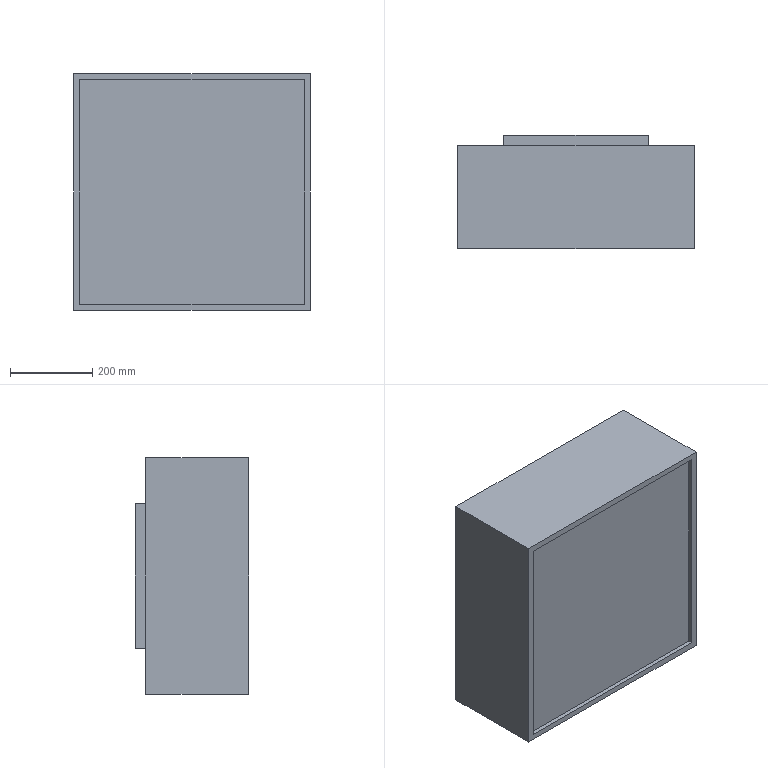Part | STEP file | FFU | 1 solid | 16 faces | box 575 x 275 x 575 mm | volume 82748500 mm3 | plane 16
STEP:
#1=CARTESIAN_POINT('',(0.,0.,0.));
#2=DIRECTION('',(0.,0.,1.));
#3=DIRECTION('',(1.,0.,0.));
#4=AXIS2_PLACEMENT_3D('',#1,#2,#3);
#5=CARTESIAN_POINT('',(-287.5,0.,-287.5));
#6=VERTEX_POINT('',#5);
#7=CARTESIAN_POINT('',(-287.5,0.,287.5));
#8=VERTEX_POINT('',#7);
#9=CARTESIAN_POINT('',(-287.5,0.,-287.5));
#10=DIRECTION('',(0.,0.,1.));
#11=VECTOR('',#10,1.);
#12=LINE('',#9,#11);
#13=CARTESIAN_POINT('',(-287.5,250.,-287.5));
#14=DIRECTION('',(1.,0.,0.));
#15=DIRECTION('',(0.,0.,-1.));
#16=AXIS2_PLACEMENT_3D('',#13,#14,#15);
#17=PLANE('',#16);
#18=CARTESIAN_POINT('',(0.,-250.));
#19=DIRECTION('',(-1.,0.));
#20=VECTOR('',#19,1.);
#21=LINE('',#18,#20);
#22=(GEOMETRIC_REPRESENTATION_CONTEXT(2)PARAMETRIC_REPRESENTATION_CONTEXT()REPRESENTATION_CONTEXT('',''));
#23=DEFINITIONAL_REPRESENTATION('',(#21),#22);
#24=PCURVE('',#17,#23);
#25=CARTESIAN_POINT('',(0.,0.,0.));
#26=DIRECTION('',(0.,1.,0.));
#27=DIRECTION('',(0.,0.,1.));
#28=AXIS2_PLACEMENT_3D('',#25,#26,#27);
#29=PLANE('',#28);
#30=CARTESIAN_POINT('',(-287.5,-287.5));
#31=DIRECTION('',(1.,0.));
#32=VECTOR('',#31,1.);
#33=LINE('',#30,#32);
#34=(GEOMETRIC_REPRESENTATION_CONTEXT(2)PARAMETRIC_REPRESENTATION_CONTEXT()REPRESENTATION_CONTEXT('',''));
#35=DEFINITIONAL_REPRESENTATION('',(#33),#34);
#36=PCURVE('',#29,#35);
#37=SURFACE_CURVE('',#12,(#24,#36),.PCURVE_S1.);
#38=EDGE_CURVE('',#6,#8,#37,.T.);
#39=ORIENTED_EDGE('',*,*,#38,.T.);
#40=CARTESIAN_POINT('',(-287.5,250.,287.5));
#41=VERTEX_POINT('',#40);
#42=CARTESIAN_POINT('',(-287.5,250.,287.5));
#43=DIRECTION('',(0.,-1.,0.));
#44=VECTOR('',#43,1.);
#45=LINE('',#42,#44);
#46=CARTESIAN_POINT('',(-575.,0.));
#47=DIRECTION('',(0.,-1.));
#48=VECTOR('',#47,1.);
#49=LINE('',#46,#48);
#50=(GEOMETRIC_REPRESENTATION_CONTEXT(2)PARAMETRIC_REPRESENTATION_CONTEXT()REPRESENTATION_CONTEXT('',''));
#51=DEFINITIONAL_REPRESENTATION('',(#49),#50);
#52=PCURVE('',#17,#51);
#53=CARTESIAN_POINT('',(-287.5,250.,287.5));
#54=DIRECTION('',(0.,0.,-1.));
#55=DIRECTION('',(-1.,0.,0.));
#56=AXIS2_PLACEMENT_3D('',#53,#54,#55);
#57=PLANE('',#56);
#58=CARTESIAN_POINT('',(0.,0.));
#59=DIRECTION('',(0.,-1.));
#60=VECTOR('',#59,1.);
#61=LINE('',#58,#60);
#62=(GEOMETRIC_REPRESENTATION_CONTEXT(2)PARAMETRIC_REPRESENTATION_CONTEXT()REPRESENTATION_CONTEXT('',''));
#63=DEFINITIONAL_REPRESENTATION('',(#61),#62);
#64=PCURVE('',#57,#63);
#65=SURFACE_CURVE('',#45,(#52,#64),.PCURVE_S1.);
#66=EDGE_CURVE('',#41,#8,#65,.T.);
#67=ORIENTED_EDGE('',*,*,#66,.F.);
#68=CARTESIAN_POINT('',(-287.5,250.,-287.5));
#69=VERTEX_POINT('',#68);
#70=CARTESIAN_POINT('',(-287.5,250.,-287.5));
#71=DIRECTION('',(0.,0.,1.));
#72=VECTOR('',#71,1.);
#73=LINE('',#70,#72);
#74=CARTESIAN_POINT('',(0.,0.));
#75=DIRECTION('',(-1.,0.));
#76=VECTOR('',#75,1.);
#77=LINE('',#74,#76);
#78=(GEOMETRIC_REPRESENTATION_CONTEXT(2)PARAMETRIC_REPRESENTATION_CONTEXT()REPRESENTATION_CONTEXT('',''));
#79=DEFINITIONAL_REPRESENTATION('',(#77),#78);
#80=PCURVE('',#17,#79);
#81=CARTESIAN_POINT('',(0.,250.,0.));
#82=DIRECTION('',(0.,1.,0.));
#83=DIRECTION('',(0.,0.,1.));
#84=AXIS2_PLACEMENT_3D('',#81,#82,#83);
#85=PLANE('',#84);
#86=CARTESIAN_POINT('',(-287.5,-287.5));
#87=DIRECTION('',(1.,0.));
#88=VECTOR('',#87,1.);
#89=LINE('',#86,#88);
#90=(GEOMETRIC_REPRESENTATION_CONTEXT(2)PARAMETRIC_REPRESENTATION_CONTEXT()REPRESENTATION_CONTEXT('',''));
#91=DEFINITIONAL_REPRESENTATION('',(#89),#90);
#92=PCURVE('',#85,#91);
#93=SURFACE_CURVE('',#73,(#80,#92),.PCURVE_S1.);
#94=EDGE_CURVE('',#69,#41,#93,.T.);
#95=ORIENTED_EDGE('',*,*,#94,.F.);
#96=CARTESIAN_POINT('',(-287.5,250.,-287.5));
#97=DIRECTION('',(0.,-1.,0.));
#98=VECTOR('',#97,1.);
#99=LINE('',#96,#98);
#100=CARTESIAN_POINT('',(0.,0.));
#101=DIRECTION('',(0.,-1.));
#102=VECTOR('',#101,1.);
#103=LINE('',#100,#102);
#104=(GEOMETRIC_REPRESENTATION_CONTEXT(2)PARAMETRIC_REPRESENTATION_CONTEXT()REPRESENTATION_CONTEXT('',''));
#105=DEFINITIONAL_REPRESENTATION('',(#103),#104);
#106=PCURVE('',#17,#105);
#107=CARTESIAN_POINT('',(-287.5,250.,-287.5));
#108=DIRECTION('',(0.,0.,1.));
#109=DIRECTION('',(1.,0.,0.));
#110=AXIS2_PLACEMENT_3D('',#107,#108,#109);
#111=PLANE('',#110);
#112=CARTESIAN_POINT('',(0.,0.));
#113=DIRECTION('',(0.,-1.));
#114=VECTOR('',#113,1.);
#115=LINE('',#112,#114);
#116=(GEOMETRIC_REPRESENTATION_CONTEXT(2)PARAMETRIC_REPRESENTATION_CONTEXT()REPRESENTATION_CONTEXT('',''));
#117=DEFINITIONAL_REPRESENTATION('',(#115),#116);
#118=PCURVE('',#111,#117);
#119=SURFACE_CURVE('',#99,(#106,#118),.PCURVE_S1.);
#120=EDGE_CURVE('',#69,#6,#119,.T.);
#121=ORIENTED_EDGE('',*,*,#120,.T.);
#122=EDGE_LOOP('',(#39,#67,#95,#121));
#123=FACE_BOUND('',#122,.T.);
#124=ADVANCED_FACE('',(#123),#17,.F.);
#125=CARTESIAN_POINT('',(287.5,0.,287.5));
#126=VERTEX_POINT('',#125);
#127=CARTESIAN_POINT('',(-287.5,0.,287.5));
#128=DIRECTION('',(1.,0.,0.));
#129=VECTOR('',#128,1.);
#130=LINE('',#127,#129);
#131=CARTESIAN_POINT('',(0.,-250.));
#132=DIRECTION('',(-1.,0.));
#133=VECTOR('',#132,1.);
#134=LINE('',#131,#133);
#135=(GEOMETRIC_REPRESENTATION_CONTEXT(2)PARAMETRIC_REPRESENTATION_CONTEXT()REPRESENTATION_CONTEXT('',''));
#136=DEFINITIONAL_REPRESENTATION('',(#134),#135);
#137=PCURVE('',#57,#136);
#138=CARTESIAN_POINT('',(287.5,-287.5));
#139=DIRECTION('',(0.,1.));
#140=VECTOR('',#139,1.);
#141=LINE('',#138,#140);
#142=(GEOMETRIC_REPRESENTATION_CONTEXT(2)PARAMETRIC_REPRESENTATION_CONTEXT()REPRESENTATION_CONTEXT('',''));
#143=DEFINITIONAL_REPRESENTATION('',(#141),#142);
#144=PCURVE('',#29,#143);
#145=SURFACE_CURVE('',#130,(#137,#144),.PCURVE_S1.);
#146=EDGE_CURVE('',#8,#126,#145,.T.);
#147=ORIENTED_EDGE('',*,*,#146,.T.);
#148=CARTESIAN_POINT('',(287.5,250.,287.5));
#149=VERTEX_POINT('',#148);
#150=CARTESIAN_POINT('',(287.5,250.,287.5));
#151=DIRECTION('',(0.,-1.,0.));
#152=VECTOR('',#151,1.);
#153=LINE('',#150,#152);
#154=CARTESIAN_POINT('',(-575.,0.));
#155=DIRECTION('',(0.,-1.));
#156=VECTOR('',#155,1.);
#157=LINE('',#154,#156);
#158=(GEOMETRIC_REPRESENTATION_CONTEXT(2)PARAMETRIC_REPRESENTATION_CONTEXT()REPRESENTATION_CONTEXT('',''));
#159=DEFINITIONAL_REPRESENTATION('',(#157),#158);
#160=PCURVE('',#57,#159);
#161=CARTESIAN_POINT('',(287.5,250.,-287.5));
#162=DIRECTION('',(-1.,0.,0.));
#163=DIRECTION('',(0.,0.,1.));
#164=AXIS2_PLACEMENT_3D('',#161,#162,#163);
#165=PLANE('',#164);
#166=CARTESIAN_POINT('',(575.,0.));
#167=DIRECTION('',(0.,-1.));
#168=VECTOR('',#167,1.);
#169=LINE('',#166,#168);
#170=(GEOMETRIC_REPRESENTATION_CONTEXT(2)PARAMETRIC_REPRESENTATION_CONTEXT()REPRESENTATION_CONTEXT('',''));
#171=DEFINITIONAL_REPRESENTATION('',(#169),#170);
#172=PCURVE('',#165,#171);
#173=SURFACE_CURVE('',#153,(#160,#172),.PCURVE_S1.);
#174=EDGE_CURVE('',#149,#126,#173,.T.);
#175=ORIENTED_EDGE('',*,*,#174,.F.);
#176=CARTESIAN_POINT('',(-287.5,250.,287.5));
#177=DIRECTION('',(1.,0.,0.));
#178=VECTOR('',#177,1.);
#179=LINE('',#176,#178);
#180=CARTESIAN_POINT('',(0.,0.));
#181=DIRECTION('',(-1.,0.));
#182=VECTOR('',#181,1.);
#183=LINE('',#180,#182);
#184=(GEOMETRIC_REPRESENTATION_CONTEXT(2)PARAMETRIC_REPRESENTATION_CONTEXT()REPRESENTATION_CONTEXT('',''));
#185=DEFINITIONAL_REPRESENTATION('',(#183),#184);
#186=PCURVE('',#57,#185);
#187=CARTESIAN_POINT('',(287.5,-287.5));
#188=DIRECTION('',(0.,1.));
#189=VECTOR('',#188,1.);
#190=LINE('',#187,#189);
#191=(GEOMETRIC_REPRESENTATION_CONTEXT(2)PARAMETRIC_REPRESENTATION_CONTEXT()REPRESENTATION_CONTEXT('',''));
#192=DEFINITIONAL_REPRESENTATION('',(#190),#191);
#193=PCURVE('',#85,#192);
#194=SURFACE_CURVE('',#179,(#186,#193),.PCURVE_S1.);
#195=EDGE_CURVE('',#41,#149,#194,.T.);
#196=ORIENTED_EDGE('',*,*,#195,.F.);
#197=ORIENTED_EDGE('',*,*,#66,.T.);
#198=EDGE_LOOP('',(#147,#175,#196,#197));
#199=FACE_BOUND('',#198,.T.);
#200=ADVANCED_FACE('',(#199),#57,.F.);
#201=CARTESIAN_POINT('',(287.5,0.,-287.5));
#202=VERTEX_POINT('',#201);
#203=CARTESIAN_POINT('',(287.5,0.,-287.5));
#204=DIRECTION('',(0.,0.,-1.));
#205=VECTOR('',#204,1.);
#206=LINE('',#203,#205);
#207=CARTESIAN_POINT('',(0.,-250.));
#208=DIRECTION('',(-1.,0.));
#209=VECTOR('',#208,1.);
#210=LINE('',#207,#209);
#211=(GEOMETRIC_REPRESENTATION_CONTEXT(2)PARAMETRIC_REPRESENTATION_CONTEXT()REPRESENTATION_CONTEXT('',''));
#212=DEFINITIONAL_REPRESENTATION('',(#210),#211);
#213=PCURVE('',#165,#212);
#214=CARTESIAN_POINT('',(-287.5,287.5));
#215=DIRECTION('',(-1.,0.));
#216=VECTOR('',#215,1.);
#217=LINE('',#214,#216);
#218=(GEOMETRIC_REPRESENTATION_CONTEXT(2)PARAMETRIC_REPRESENTATION_CONTEXT()REPRESENTATION_CONTEXT('',''));
#219=DEFINITIONAL_REPRESENTATION('',(#217),#218);
#220=PCURVE('',#29,#219);
#221=SURFACE_CURVE('',#206,(#213,#220),.PCURVE_S1.);
#222=EDGE_CURVE('',#126,#202,#221,.T.);
#223=ORIENTED_EDGE('',*,*,#222,.T.);
#224=CARTESIAN_POINT('',(287.5,250.,-287.5));
#225=VERTEX_POINT('',#224);
#226=CARTESIAN_POINT('',(287.5,250.,-287.5));
#227=DIRECTION('',(0.,-1.,0.));
#228=VECTOR('',#227,1.);
#229=LINE('',#226,#228);
#230=CARTESIAN_POINT('',(0.,0.));
#231=DIRECTION('',(0.,-1.));
#232=VECTOR('',#231,1.);
#233=LINE('',#230,#232);
#234=(GEOMETRIC_REPRESENTATION_CONTEXT(2)PARAMETRIC_REPRESENTATION_CONTEXT()REPRESENTATION_CONTEXT('',''));
#235=DEFINITIONAL_REPRESENTATION('',(#233),#234);
#236=PCURVE('',#165,#235);
#237=CARTESIAN_POINT('',(575.,0.));
#238=DIRECTION('',(0.,-1.));
#239=VECTOR('',#238,1.);
#240=LINE('',#237,#239);
#241=(GEOMETRIC_REPRESENTATION_CONTEXT(2)PARAMETRIC_REPRESENTATION_CONTEXT()REPRESENTATION_CONTEXT('',''));
#242=DEFINITIONAL_REPRESENTATION('',(#240),#241);
#243=PCURVE('',#111,#242);
#244=SURFACE_CURVE('',#229,(#236,#243),.PCURVE_S1.);
#245=EDGE_CURVE('',#225,#202,#244,.T.);
#246=ORIENTED_EDGE('',*,*,#245,.F.);
#247=CARTESIAN_POINT('',(287.5,250.,-287.5));
#248=DIRECTION('',(0.,0.,-1.));
#249=VECTOR('',#248,1.);
#250=LINE('',#247,#249);
#251=CARTESIAN_POINT('',(0.,0.));
#252=DIRECTION('',(-1.,0.));
#253=VECTOR('',#252,1.);
#254=LINE('',#251,#253);
#255=(GEOMETRIC_REPRESENTATION_CONTEXT(2)PARAMETRIC_REPRESENTATION_CONTEXT()REPRESENTATION_CONTEXT('',''));
#256=DEFINITIONAL_REPRESENTATION('',(#254),#255);
#257=PCURVE('',#165,#256);
#258=CARTESIAN_POINT('',(-287.5,287.5));
#259=DIRECTION('',(-1.,0.));
#260=VECTOR('',#259,1.);
#261=LINE('',#258,#260);
#262=(GEOMETRIC_REPRESENTATION_CONTEXT(2)PARAMETRIC_REPRESENTATION_CONTEXT()REPRESENTATION_CONTEXT('',''));
#263=DEFINITIONAL_REPRESENTATION('',(#261),#262);
#264=PCURVE('',#85,#263);
#265=SURFACE_CURVE('',#250,(#257,#264),.PCURVE_S1.);
#266=EDGE_CURVE('',#149,#225,#265,.T.);
#267=ORIENTED_EDGE('',*,*,#266,.F.);
#268=ORIENTED_EDGE('',*,*,#174,.T.);
#269=EDGE_LOOP('',(#223,#246,#267,#268));
#270=FACE_BOUND('',#269,.T.);
#271=ADVANCED_FACE('',(#270),#165,.F.);
#272=CARTESIAN_POINT('',(-287.5,0.,-287.5));
#273=DIRECTION('',(-1.,0.,0.));
#274=VECTOR('',#273,1.);
#275=LINE('',#272,#274);
#276=CARTESIAN_POINT('',(0.,-250.));
#277=DIRECTION('',(-1.,0.));
#278=VECTOR('',#277,1.);
#279=LINE('',#276,#278);
#280=(GEOMETRIC_REPRESENTATION_CONTEXT(2)PARAMETRIC_REPRESENTATION_CONTEXT()REPRESENTATION_CONTEXT('',''));
#281=DEFINITIONAL_REPRESENTATION('',(#279),#280);
#282=PCURVE('',#111,#281);
#283=CARTESIAN_POINT('',(-287.5,-287.5));
#284=DIRECTION('',(0.,-1.));
#285=VECTOR('',#284,1.);
#286=LINE('',#283,#285);
#287=(GEOMETRIC_REPRESENTATION_CONTEXT(2)PARAMETRIC_REPRESENTATION_CONTEXT()REPRESENTATION_CONTEXT('',''));
#288=DEFINITIONAL_REPRESENTATION('',(#286),#287);
#289=PCURVE('',#29,#288);
#290=SURFACE_CURVE('',#275,(#282,#289),.PCURVE_S1.);
#291=EDGE_CURVE('',#202,#6,#290,.T.);
#292=ORIENTED_EDGE('',*,*,#291,.T.);
#293=ORIENTED_EDGE('',*,*,#120,.F.);
#294=CARTESIAN_POINT('',(-287.5,250.,-287.5));
#295=DIRECTION('',(-1.,0.,0.));
#296=VECTOR('',#295,1.);
#297=LINE('',#294,#296);
#298=CARTESIAN_POINT('',(0.,0.));
#299=DIRECTION('',(-1.,0.));
#300=VECTOR('',#299,1.);
#301=LINE('',#298,#300);
#302=(GEOMETRIC_REPRESENTATION_CONTEXT(2)PARAMETRIC_REPRESENTATION_CONTEXT()REPRESENTATION_CONTEXT('',''));
#303=DEFINITIONAL_REPRESENTATION('',(#301),#302);
#304=PCURVE('',#111,#303);
#305=CARTESIAN_POINT('',(-287.5,-287.5));
#306=DIRECTION('',(0.,-1.));
#307=VECTOR('',#306,1.);
#308=LINE('',#305,#307);
#309=(GEOMETRIC_REPRESENTATION_CONTEXT(2)PARAMETRIC_REPRESENTATION_CONTEXT()REPRESENTATION_CONTEXT('',''));
#310=DEFINITIONAL_REPRESENTATION('',(#308),#309);
#311=PCURVE('',#85,#310);
#312=SURFACE_CURVE('',#297,(#304,#311),.PCURVE_S1.);
#313=EDGE_CURVE('',#225,#69,#312,.T.);
#314=ORIENTED_EDGE('',*,*,#313,.F.);
#315=ORIENTED_EDGE('',*,*,#245,.T.);
#316=EDGE_LOOP('',(#292,#293,#314,#315));
#317=FACE_BOUND('',#316,.T.);
#318=ADVANCED_FACE('',(#317),#111,.F.);
#319=CARTESIAN_POINT('',(175.,250.,175.));
#320=VERTEX_POINT('',#319);
#321=CARTESIAN_POINT('',(175.,250.,-175.));
#322=VERTEX_POINT('',#321);
#323=CARTESIAN_POINT('',(175.,250.,175.));
#324=DIRECTION('',(0.,0.,-1.));
#325=VECTOR('',#324,1.);
#326=LINE('',#323,#325);
#327=CARTESIAN_POINT('',(175.,175.));
#328=DIRECTION('',(-1.,0.));
#329=VECTOR('',#328,1.);
#330=LINE('',#327,#329);
#331=(GEOMETRIC_REPRESENTATION_CONTEXT(2)PARAMETRIC_REPRESENTATION_CONTEXT()REPRESENTATION_CONTEXT('',''));
#332=DEFINITIONAL_REPRESENTATION('',(#330),#331);
#333=PCURVE('',#85,#332);
#334=CARTESIAN_POINT('',(175.,275.,175.));
#335=DIRECTION('',(-1.,0.,0.));
#336=DIRECTION('',(0.,0.,1.));
#337=AXIS2_PLACEMENT_3D('',#334,#335,#336);
#338=PLANE('',#337);
#339=CARTESIAN_POINT('',(0.,-25.));
#340=DIRECTION('',(-1.,0.));
#341=VECTOR('',#340,1.);
#342=LINE('',#339,#341);
#343=(GEOMETRIC_REPRESENTATION_CONTEXT(2)PARAMETRIC_REPRESENTATION_CONTEXT()REPRESENTATION_CONTEXT('',''));
#344=DEFINITIONAL_REPRESENTATION('',(#342),#343);
#345=PCURVE('',#338,#344);
#346=SURFACE_CURVE('',#326,(#333,#345),.PCURVE_S1.);
#347=EDGE_CURVE('',#320,#322,#346,.T.);
#348=ORIENTED_EDGE('',*,*,#347,.F.);
#349=CARTESIAN_POINT('',(-175.,250.,175.));
#350=VERTEX_POINT('',#349);
#351=CARTESIAN_POINT('',(-175.,250.,175.));
#352=DIRECTION('',(1.,0.,0.));
#353=VECTOR('',#352,1.);
#354=LINE('',#351,#353);
#355=CARTESIAN_POINT('',(175.,-175.));
#356=DIRECTION('',(0.,1.));
#357=VECTOR('',#356,1.);
#358=LINE('',#355,#357);
#359=(GEOMETRIC_REPRESENTATION_CONTEXT(2)PARAMETRIC_REPRESENTATION_CONTEXT()REPRESENTATION_CONTEXT('',''));
#360=DEFINITIONAL_REPRESENTATION('',(#358),#359);
#361=PCURVE('',#85,#360);
#362=CARTESIAN_POINT('',(-175.,275.,175.));
#363=DIRECTION('',(0.,0.,-1.));
#364=DIRECTION('',(0.,1.,0.));
#365=AXIS2_PLACEMENT_3D('',#362,#363,#364);
#366=PLANE('',#365);
#367=CARTESIAN_POINT('',(-25.,0.));
#368=DIRECTION('',(0.,1.));
#369=VECTOR('',#368,1.);
#370=LINE('',#367,#369);
#371=(GEOMETRIC_REPRESENTATION_CONTEXT(2)PARAMETRIC_REPRESENTATION_CONTEXT()REPRESENTATION_CONTEXT('',''));
#372=DEFINITIONAL_REPRESENTATION('',(#370),#371);
#373=PCURVE('',#366,#372);
#374=SURFACE_CURVE('',#354,(#361,#373),.PCURVE_S1.);
#375=EDGE_CURVE('',#350,#320,#374,.T.);
#376=ORIENTED_EDGE('',*,*,#375,.F.);
#377=CARTESIAN_POINT('',(-175.,250.,-175.));
#378=VERTEX_POINT('',#377);
#379=CARTESIAN_POINT('',(-175.,250.,175.));
#380=DIRECTION('',(0.,0.,1.));
#381=VECTOR('',#380,1.);
#382=LINE('',#379,#381);
#383=CARTESIAN_POINT('',(175.,-175.));
#384=DIRECTION('',(1.,0.));
#385=VECTOR('',#384,1.);
#386=LINE('',#383,#385);
#387=(GEOMETRIC_REPRESENTATION_CONTEXT(2)PARAMETRIC_REPRESENTATION_CONTEXT()REPRESENTATION_CONTEXT('',''));
#388=DEFINITIONAL_REPRESENTATION('',(#386),#387);
#389=PCURVE('',#85,#388);
#390=CARTESIAN_POINT('',(-175.,275.,175.));
#391=DIRECTION('',(1.,0.,0.));
#392=DIRECTION('',(0.,0.,-1.));
#393=AXIS2_PLACEMENT_3D('',#390,#391,#392);
#394=PLANE('',#393);
#395=CARTESIAN_POINT('',(0.,-25.));
#396=DIRECTION('',(-1.,0.));
#397=VECTOR('',#396,1.);
#398=LINE('',#395,#397);
#399=(GEOMETRIC_REPRESENTATION_CONTEXT(2)PARAMETRIC_REPRESENTATION_CONTEXT()REPRESENTATION_CONTEXT('',''));
#400=DEFINITIONAL_REPRESENTATION('',(#398),#399);
#401=PCURVE('',#394,#400);
#402=SURFACE_CURVE('',#382,(#389,#401),.PCURVE_S1.);
#403=EDGE_CURVE('',#378,#350,#402,.T.);
#404=ORIENTED_EDGE('',*,*,#403,.F.);
#405=CARTESIAN_POINT('',(-175.,250.,-175.));
#406=DIRECTION('',(-1.,0.,0.));
#407=VECTOR('',#406,1.);
#408=LINE('',#405,#407);
#409=CARTESIAN_POINT('',(-175.,-175.));
#410=DIRECTION('',(0.,-1.));
#411=VECTOR('',#410,1.);
#412=LINE('',#409,#411);
#413=(GEOMETRIC_REPRESENTATION_CONTEXT(2)PARAMETRIC_REPRESENTATION_CONTEXT()REPRESENTATION_CONTEXT('',''));
#414=DEFINITIONAL_REPRESENTATION('',(#412),#413);
#415=PCURVE('',#85,#414);
#416=CARTESIAN_POINT('',(-175.,275.,-175.));
#417=DIRECTION('',(0.,0.,1.));
#418=DIRECTION('',(0.,-1.,0.));
#419=AXIS2_PLACEMENT_3D('',#416,#417,#418);
#420=PLANE('',#419);
#421=CARTESIAN_POINT('',(25.,0.));
#422=DIRECTION('',(0.,-1.));
#423=VECTOR('',#422,1.);
#424=LINE('',#421,#423);
#425=(GEOMETRIC_REPRESENTATION_CONTEXT(2)PARAMETRIC_REPRESENTATION_CONTEXT()REPRESENTATION_CONTEXT('',''));
#426=DEFINITIONAL_REPRESENTATION('',(#424),#425);
#427=PCURVE('',#420,#426);
#428=SURFACE_CURVE('',#408,(#415,#427),.PCURVE_S1.);
#429=EDGE_CURVE('',#322,#378,#428,.T.);
#430=ORIENTED_EDGE('',*,*,#429,.F.);
#431=EDGE_LOOP('',(#348,#376,#404,#430));
#432=FACE_BOUND('',#431,.T.);
#433=ORIENTED_EDGE('',*,*,#94,.T.);
#434=ORIENTED_EDGE('',*,*,#195,.T.);
#435=ORIENTED_EDGE('',*,*,#266,.T.);
#436=ORIENTED_EDGE('',*,*,#313,.T.);
#437=EDGE_LOOP('',(#433,#434,#435,#436));
#438=FACE_BOUND('',#437,.T.);
#439=ADVANCED_FACE('',(#432,#438),#85,.T.);
#440=CARTESIAN_POINT('',(-272.5,0.,-272.5));
#441=VERTEX_POINT('',#440);
#442=CARTESIAN_POINT('',(272.5,0.,-272.5));
#443=VERTEX_POINT('',#442);
#444=CARTESIAN_POINT('',(-272.5,0.,-272.5));
#445=DIRECTION('',(1.,0.,0.));
#446=VECTOR('',#445,1.);
#447=LINE('',#444,#446);
#448=CARTESIAN_POINT('',(-272.5,-272.5));
#449=DIRECTION('',(0.,1.));
#450=VECTOR('',#449,1.);
#451=LINE('',#448,#450);
#452=(GEOMETRIC_REPRESENTATION_CONTEXT(2)PARAMETRIC_REPRESENTATION_CONTEXT()REPRESENTATION_CONTEXT('',''));
#453=DEFINITIONAL_REPRESENTATION('',(#451),#452);
#454=PCURVE('',#29,#453);
#455=CARTESIAN_POINT('',(-272.5,10.,-272.5));
#456=DIRECTION('',(0.,0.,-1.));
#457=DIRECTION('',(-1.,0.,0.));
#458=AXIS2_PLACEMENT_3D('',#455,#456,#457);
#459=PLANE('',#458);
#460=CARTESIAN_POINT('',(0.,-10.));
#461=DIRECTION('',(-1.,0.));
#462=VECTOR('',#461,1.);
#463=LINE('',#460,#462);
#464=(GEOMETRIC_REPRESENTATION_CONTEXT(2)PARAMETRIC_REPRESENTATION_CONTEXT()REPRESENTATION_CONTEXT('',''));
#465=DEFINITIONAL_REPRESENTATION('',(#463),#464);
#466=PCURVE('',#459,#465);
#467=SURFACE_CURVE('',#447,(#454,#466),.PCURVE_S1.);
#468=EDGE_CURVE('',#441,#443,#467,.T.);
#469=ORIENTED_EDGE('',*,*,#468,.F.);
#470=CARTESIAN_POINT('',(-272.5,0.,272.5));
#471=VERTEX_POINT('',#470);
#472=CARTESIAN_POINT('',(-272.5,0.,272.5));
#473=DIRECTION('',(0.,0.,-1.));
#474=VECTOR('',#473,1.);
#475=LINE('',#472,#474);
#476=CARTESIAN_POINT('',(272.5,-272.5));
#477=DIRECTION('',(-1.,0.));
#478=VECTOR('',#477,1.);
#479=LINE('',#476,#478);
#480=(GEOMETRIC_REPRESENTATION_CONTEXT(2)PARAMETRIC_REPRESENTATION_CONTEXT()REPRESENTATION_CONTEXT('',''));
#481=DEFINITIONAL_REPRESENTATION('',(#479),#480);
#482=PCURVE('',#29,#481);
#483=CARTESIAN_POINT('',(-272.5,10.,272.5));
#484=DIRECTION('',(-1.,0.,0.));
#485=DIRECTION('',(0.,0.,1.));
#486=AXIS2_PLACEMENT_3D('',#483,#484,#485);
#487=PLANE('',#486);
#488=CARTESIAN_POINT('',(0.,-10.));
#489=DIRECTION('',(-1.,0.));
#490=VECTOR('',#489,1.);
#491=LINE('',#488,#490);
#492=(GEOMETRIC_REPRESENTATION_CONTEXT(2)PARAMETRIC_REPRESENTATION_CONTEXT()REPRESENTATION_CONTEXT('',''));
#493=DEFINITIONAL_REPRESENTATION('',(#491),#492);
#494=PCURVE('',#487,#493);
#495=SURFACE_CURVE('',#475,(#482,#494),.PCURVE_S1.);
#496=EDGE_CURVE('',#471,#441,#495,.T.);
#497=ORIENTED_EDGE('',*,*,#496,.F.);
#498=CARTESIAN_POINT('',(272.5,0.,272.5));
#499=VERTEX_POINT('',#498);
#500=CARTESIAN_POINT('',(-272.5,0.,272.5));
#501=DIRECTION('',(-1.,0.,0.));
#502=VECTOR('',#501,1.);
#503=LINE('',#500,#502);
#504=CARTESIAN_POINT('',(272.5,-272.5));
#505=DIRECTION('',(0.,-1.));
#506=VECTOR('',#505,1.);
#507=LINE('',#504,#506);
#508=(GEOMETRIC_REPRESENTATION_CONTEXT(2)PARAMETRIC_REPRESENTATION_CONTEXT()REPRESENTATION_CONTEXT('',''));
#509=DEFINITIONAL_REPRESENTATION('',(#507),#508);
#510=PCURVE('',#29,#509);
#511=CARTESIAN_POINT('',(-272.5,10.,272.5));
#512=DIRECTION('',(0.,0.,1.));
#513=DIRECTION('',(1.,0.,0.));
#514=AXIS2_PLACEMENT_3D('',#511,#512,#513);
#515=PLANE('',#514);
#516=CARTESIAN_POINT('',(0.,-10.));
#517=DIRECTION('',(-1.,0.));
#518=VECTOR('',#517,1.);
#519=LINE('',#516,#518);
#520=(GEOMETRIC_REPRESENTATION_CONTEXT(2)PARAMETRIC_REPRESENTATION_CONTEXT()REPRESENTATION_CONTEXT('',''));
#521=DEFINITIONAL_REPRESENTATION('',(#519),#520);
#522=PCURVE('',#515,#521);
#523=SURFACE_CURVE('',#503,(#510,#522),.PCURVE_S1.);
#524=EDGE_CURVE('',#499,#471,#523,.T.);
#525=ORIENTED_EDGE('',*,*,#524,.F.);
#526=CARTESIAN_POINT('',(272.5,0.,272.5));
#527=DIRECTION('',(0.,0.,1.));
#528=VECTOR('',#527,1.);
#529=LINE('',#526,#528);
#530=CARTESIAN_POINT('',(272.5,272.5));
#531=DIRECTION('',(1.,0.));
#532=VECTOR('',#531,1.);
#533=LINE('',#530,#532);
#534=(GEOMETRIC_REPRESENTATION_CONTEXT(2)PARAMETRIC_REPRESENTATION_CONTEXT()REPRESENTATION_CONTEXT('',''));
#535=DEFINITIONAL_REPRESENTATION('',(#533),#534);
#536=PCURVE('',#29,#535);
#537=CARTESIAN_POINT('',(272.5,10.,272.5));
#538=DIRECTION('',(1.,0.,0.));
#539=DIRECTION('',(0.,0.,-1.));
#540=AXIS2_PLACEMENT_3D('',#537,#538,#539);
#541=PLANE('',#540);
#542=CARTESIAN_POINT('',(0.,-10.));
#543=DIRECTION('',(-1.,0.));
#544=VECTOR('',#543,1.);
#545=LINE('',#542,#544);
#546=(GEOMETRIC_REPRESENTATION_CONTEXT(2)PARAMETRIC_REPRESENTATION_CONTEXT()REPRESENTATION_CONTEXT('',''));
#547=DEFINITIONAL_REPRESENTATION('',(#545),#546);
#548=PCURVE('',#541,#547);
#549=SURFACE_CURVE('',#529,(#536,#548),.PCURVE_S1.);
#550=EDGE_CURVE('',#443,#499,#549,.T.);
#551=ORIENTED_EDGE('',*,*,#550,.F.);
#552=EDGE_LOOP('',(#469,#497,#525,#551));
#553=FACE_BOUND('',#552,.T.);
#554=ORIENTED_EDGE('',*,*,#38,.F.);
#555=ORIENTED_EDGE('',*,*,#291,.F.);
#556=ORIENTED_EDGE('',*,*,#222,.F.);
#557=ORIENTED_EDGE('',*,*,#146,.F.);
#558=EDGE_LOOP('',(#554,#555,#556,#557));
#559=FACE_BOUND('',#558,.T.);
#560=ADVANCED_FACE('',(#553,#559),#29,.F.);
#561=ORIENTED_EDGE('',*,*,#496,.T.);
#562=CARTESIAN_POINT('',(-272.5,10.,-272.5));
#563=VERTEX_POINT('',#562);
#564=CARTESIAN_POINT('',(-272.5,10.,-272.5));
#565=DIRECTION('',(0.,-1.,0.));
#566=VECTOR('',#565,1.);
#567=LINE('',#564,#566);
#568=CARTESIAN_POINT('',(-545.,0.));
#569=DIRECTION('',(0.,-1.));
#570=VECTOR('',#569,1.);
#571=LINE('',#568,#570);
#572=(GEOMETRIC_REPRESENTATION_CONTEXT(2)PARAMETRIC_REPRESENTATION_CONTEXT()REPRESENTATION_CONTEXT('',''));
#573=DEFINITIONAL_REPRESENTATION('',(#571),#572);
#574=PCURVE('',#487,#573);
#575=CARTESIAN_POINT('',(0.,0.));
#576=DIRECTION('',(0.,-1.));
#577=VECTOR('',#576,1.);
#578=LINE('',#575,#577);
#579=(GEOMETRIC_REPRESENTATION_CONTEXT(2)PARAMETRIC_REPRESENTATION_CONTEXT()REPRESENTATION_CONTEXT('',''));
#580=DEFINITIONAL_REPRESENTATION('',(#578),#579);
#581=PCURVE('',#459,#580);
#582=SURFACE_CURVE('',#567,(#574,#581),.PCURVE_S1.);
#583=EDGE_CURVE('',#563,#441,#582,.T.);
#584=ORIENTED_EDGE('',*,*,#583,.F.);
#585=CARTESIAN_POINT('',(-272.5,10.,272.5));
#586=VERTEX_POINT('',#585);
#587=CARTESIAN_POINT('',(-272.5,10.,272.5));
#588=DIRECTION('',(0.,0.,-1.));
#589=VECTOR('',#588,1.);
#590=LINE('',#587,#589);
#591=CARTESIAN_POINT('',(0.,0.));
#592=DIRECTION('',(-1.,0.));
#593=VECTOR('',#592,1.);
#594=LINE('',#591,#593);
#595=(GEOMETRIC_REPRESENTATION_CONTEXT(2)PARAMETRIC_REPRESENTATION_CONTEXT()REPRESENTATION_CONTEXT('',''));
#596=DEFINITIONAL_REPRESENTATION('',(#594),#595);
#597=PCURVE('',#487,#596);
#598=CARTESIAN_POINT('',(0.,10.,0.));
#599=DIRECTION('',(0.,-1.,0.));
#600=DIRECTION('',(0.,0.,-1.));
#601=AXIS2_PLACEMENT_3D('',#598,#599,#600);
#602=PLANE('',#601);
#603=CARTESIAN_POINT('',(-272.5,-272.5));
#604=DIRECTION('',(1.,0.));
#605=VECTOR('',#604,1.);
#606=LINE('',#603,#605);
#607=(GEOMETRIC_REPRESENTATION_CONTEXT(2)PARAMETRIC_REPRESENTATION_CONTEXT()REPRESENTATION_CONTEXT('',''));
#608=DEFINITIONAL_REPRESENTATION('',(#606),#607);
#609=PCURVE('',#602,#608);
#610=SURFACE_CURVE('',#590,(#597,#609),.PCURVE_S1.);
#611=EDGE_CURVE('',#586,#563,#610,.T.);
#612=ORIENTED_EDGE('',*,*,#611,.F.);
#613=CARTESIAN_POINT('',(-272.5,10.,272.5));
#614=DIRECTION('',(0.,-1.,0.));
#615=VECTOR('',#614,1.);
#616=LINE('',#613,#615);
#617=CARTESIAN_POINT('',(0.,0.));
#618=DIRECTION('',(0.,-1.));
#619=VECTOR('',#618,1.);
#620=LINE('',#617,#619);
#621=(GEOMETRIC_REPRESENTATION_CONTEXT(2)PARAMETRIC_REPRESENTATION_CONTEXT()REPRESENTATION_CONTEXT('',''));
#622=DEFINITIONAL_REPRESENTATION('',(#620),#621);
#623=PCURVE('',#487,#622);
#624=CARTESIAN_POINT('',(0.,0.));
#625=DIRECTION('',(0.,-1.));
#626=VECTOR('',#625,1.);
#627=LINE('',#624,#626);
#628=(GEOMETRIC_REPRESENTATION_CONTEXT(2)PARAMETRIC_REPRESENTATION_CONTEXT()REPRESENTATION_CONTEXT('',''));
#629=DEFINITIONAL_REPRESENTATION('',(#627),#628);
#630=PCURVE('',#515,#629);
#631=SURFACE_CURVE('',#616,(#623,#630),.PCURVE_S1.);
#632=EDGE_CURVE('',#586,#471,#631,.T.);
#633=ORIENTED_EDGE('',*,*,#632,.T.);
#634=EDGE_LOOP('',(#561,#584,#612,#633));
#635=FACE_BOUND('',#634,.T.);
#636=ADVANCED_FACE('',(#635),#487,.F.);
#637=ORIENTED_EDGE('',*,*,#524,.T.);
#638=ORIENTED_EDGE('',*,*,#632,.F.);
#639=CARTESIAN_POINT('',(272.5,10.,272.5));
#640=VERTEX_POINT('',#639);
#641=CARTESIAN_POINT('',(-272.5,10.,272.5));
#642=DIRECTION('',(-1.,0.,0.));
#643=VECTOR('',#642,1.);
#644=LINE('',#641,#643);
#645=CARTESIAN_POINT('',(0.,0.));
#646=DIRECTION('',(-1.,0.));
#647=VECTOR('',#646,1.);
#648=LINE('',#645,#647);
#649=(GEOMETRIC_REPRESENTATION_CONTEXT(2)PARAMETRIC_REPRESENTATION_CONTEXT()REPRESENTATION_CONTEXT('',''));
#650=DEFINITIONAL_REPRESENTATION('',(#648),#649);
#651=PCURVE('',#515,#650);
#652=CARTESIAN_POINT('',(-272.5,-272.5));
#653=DIRECTION('',(0.,-1.));
#654=VECTOR('',#653,1.);
#655=LINE('',#652,#654);
#656=(GEOMETRIC_REPRESENTATION_CONTEXT(2)PARAMETRIC_REPRESENTATION_CONTEXT()REPRESENTATION_CONTEXT('',''));
#657=DEFINITIONAL_REPRESENTATION('',(#655),#656);
#658=PCURVE('',#602,#657);
#659=SURFACE_CURVE('',#644,(#651,#658),.PCURVE_S1.);
#660=EDGE_CURVE('',#640,#586,#659,.T.);
#661=ORIENTED_EDGE('',*,*,#660,.F.);
#662=CARTESIAN_POINT('',(272.5,10.,272.5));
#663=DIRECTION('',(0.,-1.,0.));
#664=VECTOR('',#663,1.);
#665=LINE('',#662,#664);
#666=CARTESIAN_POINT('',(545.,0.));
#667=DIRECTION('',(0.,-1.));
#668=VECTOR('',#667,1.);
#669=LINE('',#666,#668);
#670=(GEOMETRIC_REPRESENTATION_CONTEXT(2)PARAMETRIC_REPRESENTATION_CONTEXT()REPRESENTATION_CONTEXT('',''));
#671=DEFINITIONAL_REPRESENTATION('',(#669),#670);
#672=PCURVE('',#515,#671);
#673=CARTESIAN_POINT('',(0.,0.));
#674=DIRECTION('',(0.,-1.));
#675=VECTOR('',#674,1.);
#676=LINE('',#673,#675);
#677=(GEOMETRIC_REPRESENTATION_CONTEXT(2)PARAMETRIC_REPRESENTATION_CONTEXT()REPRESENTATION_CONTEXT('',''));
#678=DEFINITIONAL_REPRESENTATION('',(#676),#677);
#679=PCURVE('',#541,#678);
#680=SURFACE_CURVE('',#665,(#672,#679),.PCURVE_S1.);
#681=EDGE_CURVE('',#640,#499,#680,.T.);
#682=ORIENTED_EDGE('',*,*,#681,.T.);
#683=EDGE_LOOP('',(#637,#638,#661,#682));
#684=FACE_BOUND('',#683,.T.);
#685=ADVANCED_FACE('',(#684),#515,.F.);
#686=ORIENTED_EDGE('',*,*,#550,.T.);
#687=ORIENTED_EDGE('',*,*,#681,.F.);
#688=CARTESIAN_POINT('',(272.5,10.,-272.5));
#689=VERTEX_POINT('',#688);
#690=CARTESIAN_POINT('',(272.5,10.,272.5));
#691=DIRECTION('',(0.,0.,1.));
#692=VECTOR('',#691,1.);
#693=LINE('',#690,#692);
#694=CARTESIAN_POINT('',(0.,0.));
#695=DIRECTION('',(-1.,0.));
#696=VECTOR('',#695,1.);
#697=LINE('',#694,#696);
#698=(GEOMETRIC_REPRESENTATION_CONTEXT(2)PARAMETRIC_REPRESENTATION_CONTEXT()REPRESENTATION_CONTEXT('',''));
#699=DEFINITIONAL_REPRESENTATION('',(#697),#698);
#700=PCURVE('',#541,#699);
#701=CARTESIAN_POINT('',(-272.5,272.5));
#702=DIRECTION('',(-1.,0.));
#703=VECTOR('',#702,1.);
#704=LINE('',#701,#703);
#705=(GEOMETRIC_REPRESENTATION_CONTEXT(2)PARAMETRIC_REPRESENTATION_CONTEXT()REPRESENTATION_CONTEXT('',''));
#706=DEFINITIONAL_REPRESENTATION('',(#704),#705);
#707=PCURVE('',#602,#706);
#708=SURFACE_CURVE('',#693,(#700,#707),.PCURVE_S1.);
#709=EDGE_CURVE('',#689,#640,#708,.T.);
#710=ORIENTED_EDGE('',*,*,#709,.F.);
#711=CARTESIAN_POINT('',(272.5,10.,-272.5));
#712=DIRECTION('',(0.,-1.,0.));
#713=VECTOR('',#712,1.);
#714=LINE('',#711,#713);
#715=CARTESIAN_POINT('',(545.,0.));
#716=DIRECTION('',(0.,-1.));
#717=VECTOR('',#716,1.);
#718=LINE('',#715,#717);
#719=(GEOMETRIC_REPRESENTATION_CONTEXT(2)PARAMETRIC_REPRESENTATION_CONTEXT()REPRESENTATION_CONTEXT('',''));
#720=DEFINITIONAL_REPRESENTATION('',(#718),#719);
#721=PCURVE('',#541,#720);
#722=CARTESIAN_POINT('',(-545.,0.));
#723=DIRECTION('',(0.,-1.));
#724=VECTOR('',#723,1.);
#725=LINE('',#722,#724);
#726=(GEOMETRIC_REPRESENTATION_CONTEXT(2)PARAMETRIC_REPRESENTATION_CONTEXT()REPRESENTATION_CONTEXT('',''));
#727=DEFINITIONAL_REPRESENTATION('',(#725),#726);
#728=PCURVE('',#459,#727);
#729=SURFACE_CURVE('',#714,(#721,#728),.PCURVE_S1.);
#730=EDGE_CURVE('',#689,#443,#729,.T.);
#731=ORIENTED_EDGE('',*,*,#730,.T.);
#732=EDGE_LOOP('',(#686,#687,#710,#731));
#733=FACE_BOUND('',#732,.T.);
#734=ADVANCED_FACE('',(#733),#541,.F.);
#735=ORIENTED_EDGE('',*,*,#468,.T.);
#736=ORIENTED_EDGE('',*,*,#730,.F.);
#737=CARTESIAN_POINT('',(-272.5,10.,-272.5));
#738=DIRECTION('',(1.,0.,0.));
#739=VECTOR('',#738,1.);
#740=LINE('',#737,#739);
#741=CARTESIAN_POINT('',(0.,0.));
#742=DIRECTION('',(-1.,0.));
#743=VECTOR('',#742,1.);
#744=LINE('',#741,#743);
#745=(GEOMETRIC_REPRESENTATION_CONTEXT(2)PARAMETRIC_REPRESENTATION_CONTEXT()REPRESENTATION_CONTEXT('',''));
#746=DEFINITIONAL_REPRESENTATION('',(#744),#745);
#747=PCURVE('',#459,#746);
#748=CARTESIAN_POINT('',(272.5,-272.5));
#749=DIRECTION('',(0.,1.));
#750=VECTOR('',#749,1.);
#751=LINE('',#748,#750);
#752=(GEOMETRIC_REPRESENTATION_CONTEXT(2)PARAMETRIC_REPRESENTATION_CONTEXT()REPRESENTATION_CONTEXT('',''));
#753=DEFINITIONAL_REPRESENTATION('',(#751),#752);
#754=PCURVE('',#602,#753);
#755=SURFACE_CURVE('',#740,(#747,#754),.PCURVE_S1.);
#756=EDGE_CURVE('',#563,#689,#755,.T.);
#757=ORIENTED_EDGE('',*,*,#756,.F.);
#758=ORIENTED_EDGE('',*,*,#583,.T.);
#759=EDGE_LOOP('',(#735,#736,#757,#758));
#760=FACE_BOUND('',#759,.T.);
#761=ADVANCED_FACE('',(#760),#459,.F.);
#762=ORIENTED_EDGE('',*,*,#611,.T.);
#763=ORIENTED_EDGE('',*,*,#756,.T.);
#764=ORIENTED_EDGE('',*,*,#709,.T.);
#765=ORIENTED_EDGE('',*,*,#660,.T.);
#766=EDGE_LOOP('',(#762,#763,#764,#765));
#767=FACE_BOUND('',#766,.T.);
#768=ADVANCED_FACE('',(#767),#602,.T.);
#769=ORIENTED_EDGE('',*,*,#347,.T.);
#770=CARTESIAN_POINT('',(175.,275.,-175.));
#771=VERTEX_POINT('',#770);
#772=CARTESIAN_POINT('',(175.,275.,-175.));
#773=DIRECTION('',(0.,-1.,0.));
#774=VECTOR('',#773,1.);
#775=LINE('',#772,#774);
#776=CARTESIAN_POINT('',(-350.,0.));
#777=DIRECTION('',(0.,-1.));
#778=VECTOR('',#777,1.);
#779=LINE('',#776,#778);
#780=(GEOMETRIC_REPRESENTATION_CONTEXT(2)PARAMETRIC_REPRESENTATION_CONTEXT()REPRESENTATION_CONTEXT('',''));
#781=DEFINITIONAL_REPRESENTATION('',(#779),#780);
#782=PCURVE('',#338,#781);
#783=CARTESIAN_POINT('',(0.,350.));
#784=DIRECTION('',(1.,0.));
#785=VECTOR('',#784,1.);
#786=LINE('',#783,#785);
#787=(GEOMETRIC_REPRESENTATION_CONTEXT(2)PARAMETRIC_REPRESENTATION_CONTEXT()REPRESENTATION_CONTEXT('',''));
#788=DEFINITIONAL_REPRESENTATION('',(#786),#787);
#789=PCURVE('',#420,#788);
#790=SURFACE_CURVE('',#775,(#782,#789),.PCURVE_S1.);
#791=EDGE_CURVE('',#771,#322,#790,.T.);
#792=ORIENTED_EDGE('',*,*,#791,.F.);
#793=CARTESIAN_POINT('',(175.,275.,175.));
#794=VERTEX_POINT('',#793);
#795=CARTESIAN_POINT('',(175.,275.,175.));
#796=DIRECTION('',(0.,0.,-1.));
#797=VECTOR('',#796,1.);
#798=LINE('',#795,#797);
#799=CARTESIAN_POINT('',(0.,0.));
#800=DIRECTION('',(-1.,0.));
#801=VECTOR('',#800,1.);
#802=LINE('',#799,#801);
#803=(GEOMETRIC_REPRESENTATION_CONTEXT(2)PARAMETRIC_REPRESENTATION_CONTEXT()REPRESENTATION_CONTEXT('',''));
#804=DEFINITIONAL_REPRESENTATION('',(#802),#803);
#805=PCURVE('',#338,#804);
#806=CARTESIAN_POINT('',(0.,275.,0.));
#807=DIRECTION('',(0.,-1.,0.));
#808=DIRECTION('',(0.,0.,-1.));
#809=AXIS2_PLACEMENT_3D('',#806,#807,#808);
#810=PLANE('',#809);
#811=CARTESIAN_POINT('',(-175.,175.));
#812=DIRECTION('',(1.,0.));
#813=VECTOR('',#812,1.);
#814=LINE('',#811,#813);
#815=(GEOMETRIC_REPRESENTATION_CONTEXT(2)PARAMETRIC_REPRESENTATION_CONTEXT()REPRESENTATION_CONTEXT('',''));
#816=DEFINITIONAL_REPRESENTATION('',(#814),#815);
#817=PCURVE('',#810,#816);
#818=SURFACE_CURVE('',#798,(#805,#817),.PCURVE_S1.);
#819=EDGE_CURVE('',#794,#771,#818,.T.);
#820=ORIENTED_EDGE('',*,*,#819,.F.);
#821=CARTESIAN_POINT('',(175.,275.,175.));
#822=DIRECTION('',(0.,-1.,0.));
#823=VECTOR('',#822,1.);
#824=LINE('',#821,#823);
#825=CARTESIAN_POINT('',(0.,0.));
#826=DIRECTION('',(0.,-1.));
#827=VECTOR('',#826,1.);
#828=LINE('',#825,#827);
#829=(GEOMETRIC_REPRESENTATION_CONTEXT(2)PARAMETRIC_REPRESENTATION_CONTEXT()REPRESENTATION_CONTEXT('',''));
#830=DEFINITIONAL_REPRESENTATION('',(#828),#829);
#831=PCURVE('',#338,#830);
#832=CARTESIAN_POINT('',(0.,350.));
#833=DIRECTION('',(-1.,0.));
#834=VECTOR('',#833,1.);
#835=LINE('',#832,#834);
#836=(GEOMETRIC_REPRESENTATION_CONTEXT(2)PARAMETRIC_REPRESENTATION_CONTEXT()REPRESENTATION_CONTEXT('',''));
#837=DEFINITIONAL_REPRESENTATION('',(#835),#836);
#838=PCURVE('',#366,#837);
#839=SURFACE_CURVE('',#824,(#831,#838),.PCURVE_S1.);
#840=EDGE_CURVE('',#794,#320,#839,.T.);
#841=ORIENTED_EDGE('',*,*,#840,.T.);
#842=EDGE_LOOP('',(#769,#792,#820,#841));
#843=FACE_BOUND('',#842,.T.);
#844=ADVANCED_FACE('',(#843),#338,.F.);
#845=ORIENTED_EDGE('',*,*,#429,.T.);
#846=CARTESIAN_POINT('',(-175.,275.,-175.));
#847=VERTEX_POINT('',#846);
#848=CARTESIAN_POINT('',(-175.,275.,-175.));
#849=DIRECTION('',(0.,-1.,0.));
#850=VECTOR('',#849,1.);
#851=LINE('',#848,#850);
#852=CARTESIAN_POINT('',(0.,0.));
#853=DIRECTION('',(1.,0.));
#854=VECTOR('',#853,1.);
#855=LINE('',#852,#854);
#856=(GEOMETRIC_REPRESENTATION_CONTEXT(2)PARAMETRIC_REPRESENTATION_CONTEXT()REPRESENTATION_CONTEXT('',''));
#857=DEFINITIONAL_REPRESENTATION('',(#855),#856);
#858=PCURVE('',#420,#857);
#859=CARTESIAN_POINT('',(350.,0.));
#860=DIRECTION('',(0.,-1.));
#861=VECTOR('',#860,1.);
#862=LINE('',#859,#861);
#863=(GEOMETRIC_REPRESENTATION_CONTEXT(2)PARAMETRIC_REPRESENTATION_CONTEXT()REPRESENTATION_CONTEXT('',''));
#864=DEFINITIONAL_REPRESENTATION('',(#862),#863);
#865=PCURVE('',#394,#864);
#866=SURFACE_CURVE('',#851,(#858,#865),.PCURVE_S1.);
#867=EDGE_CURVE('',#847,#378,#866,.T.);
#868=ORIENTED_EDGE('',*,*,#867,.F.);
#869=CARTESIAN_POINT('',(-175.,275.,-175.));
#870=DIRECTION('',(-1.,0.,0.));
#871=VECTOR('',#870,1.);
#872=LINE('',#869,#871);
#873=CARTESIAN_POINT('',(0.,0.));
#874=DIRECTION('',(0.,-1.));
#875=VECTOR('',#874,1.);
#876=LINE('',#873,#875);
#877=(GEOMETRIC_REPRESENTATION_CONTEXT(2)PARAMETRIC_REPRESENTATION_CONTEXT()REPRESENTATION_CONTEXT('',''));
#878=DEFINITIONAL_REPRESENTATION('',(#876),#877);
#879=PCURVE('',#420,#878);
#880=CARTESIAN_POINT('',(175.,-175.));
#881=DIRECTION('',(0.,-1.));
#882=VECTOR('',#881,1.);
#883=LINE('',#880,#882);
#884=(GEOMETRIC_REPRESENTATION_CONTEXT(2)PARAMETRIC_REPRESENTATION_CONTEXT()REPRESENTATION_CONTEXT('',''));
#885=DEFINITIONAL_REPRESENTATION('',(#883),#884);
#886=PCURVE('',#810,#885);
#887=SURFACE_CURVE('',#872,(#879,#886),.PCURVE_S1.);
#888=EDGE_CURVE('',#771,#847,#887,.T.);
#889=ORIENTED_EDGE('',*,*,#888,.F.);
#890=ORIENTED_EDGE('',*,*,#791,.T.);
#891=EDGE_LOOP('',(#845,#868,#889,#890));
#892=FACE_BOUND('',#891,.T.);
#893=ADVANCED_FACE('',(#892),#420,.F.);
#894=ORIENTED_EDGE('',*,*,#403,.T.);
#895=CARTESIAN_POINT('',(-175.,275.,175.));
#896=VERTEX_POINT('',#895);
#897=CARTESIAN_POINT('',(-175.,275.,175.));
#898=DIRECTION('',(0.,-1.,0.));
#899=VECTOR('',#898,1.);
#900=LINE('',#897,#899);
#901=CARTESIAN_POINT('',(0.,0.));
#902=DIRECTION('',(0.,-1.));
#903=VECTOR('',#902,1.);
#904=LINE('',#901,#903);
#905=(GEOMETRIC_REPRESENTATION_CONTEXT(2)PARAMETRIC_REPRESENTATION_CONTEXT()REPRESENTATION_CONTEXT('',''));
#906=DEFINITIONAL_REPRESENTATION('',(#904),#905);
#907=PCURVE('',#394,#906);
#908=CARTESIAN_POINT('',(0.,0.));
#909=DIRECTION('',(-1.,0.));
#910=VECTOR('',#909,1.);
#911=LINE('',#908,#910);
#912=(GEOMETRIC_REPRESENTATION_CONTEXT(2)PARAMETRIC_REPRESENTATION_CONTEXT()REPRESENTATION_CONTEXT('',''));
#913=DEFINITIONAL_REPRESENTATION('',(#911),#912);
#914=PCURVE('',#366,#913);
#915=SURFACE_CURVE('',#900,(#907,#914),.PCURVE_S1.);
#916=EDGE_CURVE('',#896,#350,#915,.T.);
#917=ORIENTED_EDGE('',*,*,#916,.F.);
#918=CARTESIAN_POINT('',(-175.,275.,175.));
#919=DIRECTION('',(0.,0.,1.));
#920=VECTOR('',#919,1.);
#921=LINE('',#918,#920);
#922=CARTESIAN_POINT('',(0.,0.));
#923=DIRECTION('',(-1.,0.));
#924=VECTOR('',#923,1.);
#925=LINE('',#922,#924);
#926=(GEOMETRIC_REPRESENTATION_CONTEXT(2)PARAMETRIC_REPRESENTATION_CONTEXT()REPRESENTATION_CONTEXT('',''));
#927=DEFINITIONAL_REPRESENTATION('',(#925),#926);
#928=PCURVE('',#394,#927);
#929=CARTESIAN_POINT('',(-175.,-175.));
#930=DIRECTION('',(-1.,0.));
#931=VECTOR('',#930,1.);
#932=LINE('',#929,#931);
#933=(GEOMETRIC_REPRESENTATION_CONTEXT(2)PARAMETRIC_REPRESENTATION_CONTEXT()REPRESENTATION_CONTEXT('',''));
#934=DEFINITIONAL_REPRESENTATION('',(#932),#933);
#935=PCURVE('',#810,#934);
#936=SURFACE_CURVE('',#921,(#928,#935),.PCURVE_S1.);
#937=EDGE_CURVE('',#847,#896,#936,.T.);
#938=ORIENTED_EDGE('',*,*,#937,.F.);
#939=ORIENTED_EDGE('',*,*,#867,.T.);
#940=EDGE_LOOP('',(#894,#917,#938,#939));
#941=FACE_BOUND('',#940,.T.);
#942=ADVANCED_FACE('',(#941),#394,.F.);
#943=ORIENTED_EDGE('',*,*,#375,.T.);
#944=ORIENTED_EDGE('',*,*,#840,.F.);
#945=CARTESIAN_POINT('',(-175.,275.,175.));
#946=DIRECTION('',(1.,0.,0.));
#947=VECTOR('',#946,1.);
#948=LINE('',#945,#947);
#949=CARTESIAN_POINT('',(0.,0.));
#950=DIRECTION('',(0.,1.));
#951=VECTOR('',#950,1.);
#952=LINE('',#949,#951);
#953=(GEOMETRIC_REPRESENTATION_CONTEXT(2)PARAMETRIC_REPRESENTATION_CONTEXT()REPRESENTATION_CONTEXT('',''));
#954=DEFINITIONAL_REPRESENTATION('',(#952),#953);
#955=PCURVE('',#366,#954);
#956=CARTESIAN_POINT('',(-175.,-175.));
#957=DIRECTION('',(0.,1.));
#958=VECTOR('',#957,1.);
#959=LINE('',#956,#958);
#960=(GEOMETRIC_REPRESENTATION_CONTEXT(2)PARAMETRIC_REPRESENTATION_CONTEXT()REPRESENTATION_CONTEXT('',''));
#961=DEFINITIONAL_REPRESENTATION('',(#959),#960);
#962=PCURVE('',#810,#961);
#963=SURFACE_CURVE('',#948,(#955,#962),.PCURVE_S1.);
#964=EDGE_CURVE('',#896,#794,#963,.T.);
#965=ORIENTED_EDGE('',*,*,#964,.F.);
#966=ORIENTED_EDGE('',*,*,#916,.T.);
#967=EDGE_LOOP('',(#943,#944,#965,#966));
#968=FACE_BOUND('',#967,.T.);
#969=ADVANCED_FACE('',(#968),#366,.F.);
#970=ORIENTED_EDGE('',*,*,#819,.T.);
#971=ORIENTED_EDGE('',*,*,#888,.T.);
#972=ORIENTED_EDGE('',*,*,#937,.T.);
#973=ORIENTED_EDGE('',*,*,#964,.T.);
#974=EDGE_LOOP('',(#970,#971,#972,#973));
#975=FACE_BOUND('',#974,.T.);
#976=ADVANCED_FACE('',(#975),#810,.F.);
#977=CLOSED_SHELL('',(#124,#200,#271,#318,#439,#560,#636,#685,#734,#761,#768,#844,#893,#942,#969,#976));
#978=MANIFOLD_SOLID_BREP('',#977);
#979=(LENGTH_UNIT()NAMED_UNIT(*)SI_UNIT(.MILLI.,.METRE.));
#980=UNCERTAINTY_MEASURE_WITH_UNIT(LENGTH_MEASURE(0.0000001),#979,'','');
#981=(NAMED_UNIT(*)PLANE_ANGLE_UNIT()SI_UNIT($,.RADIAN.));
#982=(NAMED_UNIT(*)SI_UNIT($,.STERADIAN.)SOLID_ANGLE_UNIT());
#983=(GEOMETRIC_REPRESENTATION_CONTEXT(3)GLOBAL_UNCERTAINTY_ASSIGNED_CONTEXT((#980))GLOBAL_UNIT_ASSIGNED_CONTEXT((#979,#981,#982))REPRESENTATION_CONTEXT('',''));
#984=ADVANCED_BREP_SHAPE_REPRESENTATION('',(#4,#978),#983);